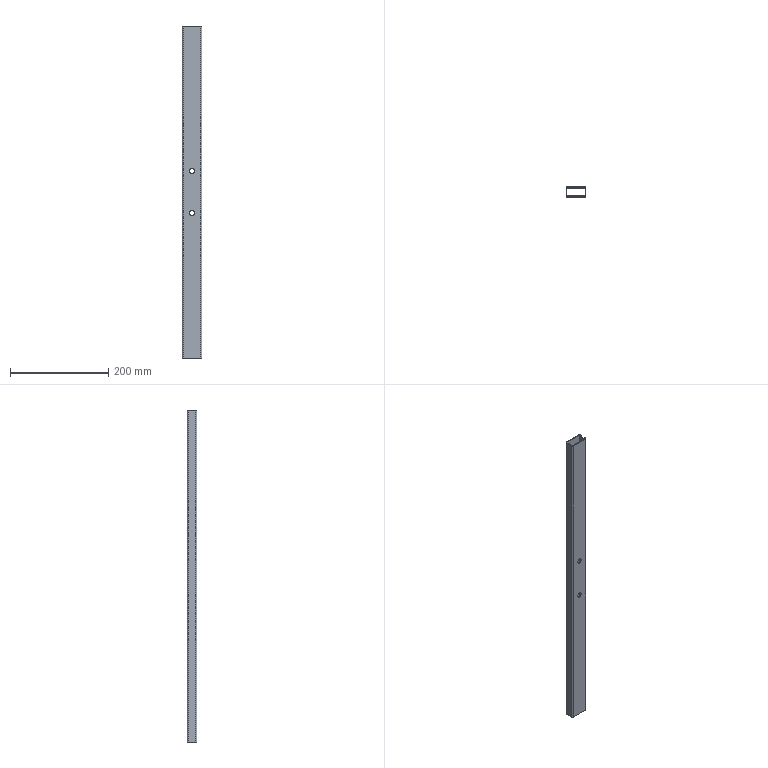Part | STEP file | 6100102 | 1 solid | 24 faces | box 40 x 20 x 675 mm | volume 111794 mm3 | cylinder 14 | plane 10 | commonest cylinder face diameters 10 x6 2 x4 5 x4